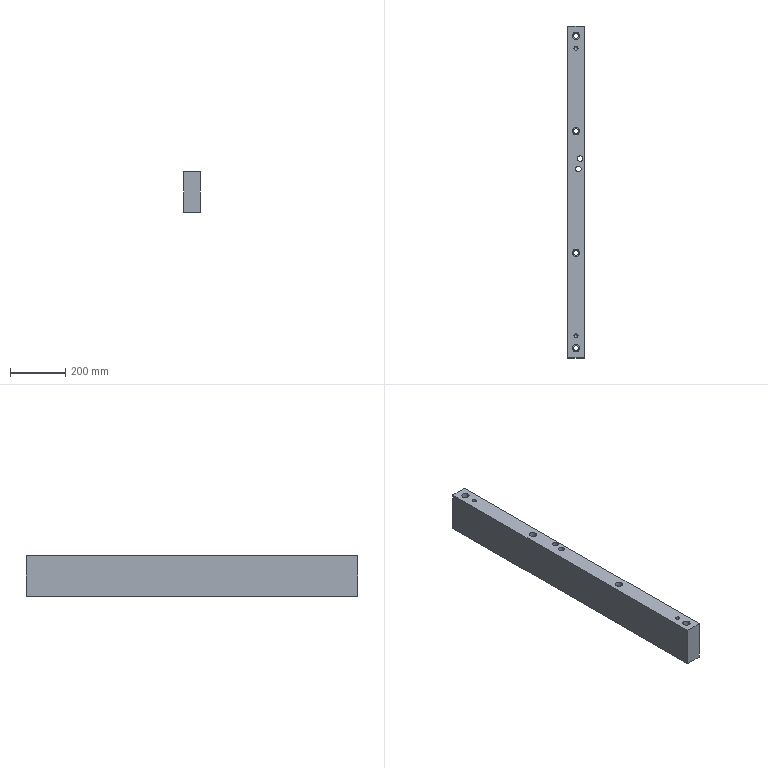Part | STEP file | lll_id2474_x_t | 1 solid | 24 faces | box 60 x 1200 x 147.5 mm | volume 10289095 mm3 | cylinder 12 | plane 10 | cone 2 | commonest cylinder face diameters 18.009 x4 26.008 x4 14.506 x2 20 x2
STEP:
#1=CARTESIAN_POINT('',(777.004,120.5,222.5));
#2=VERTEX_POINT('',#1);
#3=CARTESIAN_POINT('',(767.004,120.5,222.5));
#4=DIRECTION('',(0.,0.,1.));
#5=DIRECTION('',(1.,0.,0.));
#6=AXIS2_PLACEMENT_3D('',#3,#4,#5);
#7=CIRCLE('',#6,10.);
#8=EDGE_CURVE('',#2,#2,#7,.T.);
#9=ORIENTED_EDGE('',*,*,#8,.T.);
#10=EDGE_LOOP('',(#9));
#11=FACE_BOUND('',#10,.T.);
#12=CARTESIAN_POINT('',(761.44,-220.,222.5));
#13=VERTEX_POINT('',#12);
#14=CARTESIAN_POINT('',(752.435,-220.,222.5));
#15=DIRECTION('',(0.,0.,1.));
#16=DIRECTION('',(1.,0.,0.));
#17=AXIS2_PLACEMENT_3D('',#14,#15,#16);
#18=CIRCLE('',#17,9.005);
#19=EDGE_CURVE('',#13,#13,#18,.T.);
#20=ORIENTED_EDGE('',*,*,#19,.T.);
#21=EDGE_LOOP('',(#20));
#22=FACE_BOUND('',#21,.T.);
#23=CARTESIAN_POINT('',(722.435,600.,222.5));
#24=VERTEX_POINT('',#23);
#25=CARTESIAN_POINT('',(782.435,600.,222.5));
#26=VERTEX_POINT('',#25);
#27=CARTESIAN_POINT('',(-3187.565,600.,222.5));
#28=DIRECTION('',(1.,0.,0.));
#29=VECTOR('',#28,1.);
#30=LINE('',#27,#29);
#31=EDGE_CURVE('',#24,#26,#30,.T.);
#32=ORIENTED_EDGE('',*,*,#31,.T.);
#33=CARTESIAN_POINT('',(782.435,-600.,222.5));
#34=VERTEX_POINT('',#33);
#35=CARTESIAN_POINT('',(782.435,600.,222.5));
#36=DIRECTION('',(0.,-1.,0.));
#37=VECTOR('',#36,1.);
#38=LINE('',#35,#37);
#39=EDGE_CURVE('',#26,#34,#38,.T.);
#40=ORIENTED_EDGE('',*,*,#39,.T.);
#41=CARTESIAN_POINT('',(722.435,-600.,222.5));
#42=VERTEX_POINT('',#41);
#43=CARTESIAN_POINT('',(782.435,-600.,222.5));
#44=DIRECTION('',(-1.,0.,0.));
#45=VECTOR('',#44,1.);
#46=LINE('',#43,#45);
#47=EDGE_CURVE('',#34,#42,#46,.T.);
#48=ORIENTED_EDGE('',*,*,#47,.T.);
#49=CARTESIAN_POINT('',(722.435,1.,222.5));
#50=DIRECTION('',(0.,-1.,0.));
#51=VECTOR('',#50,1.);
#52=LINE('',#49,#51);
#53=EDGE_CURVE('',#24,#42,#52,.T.);
#54=ORIENTED_EDGE('',*,*,#53,.F.);
#55=EDGE_LOOP('',(#32,#40,#48,#54));
#56=FACE_BOUND('',#55,.T.);
#57=CARTESIAN_POINT('',(761.44,-565.,222.5));
#58=VERTEX_POINT('',#57);
#59=CARTESIAN_POINT('',(752.435,-565.,222.5));
#60=DIRECTION('',(0.,0.,1.));
#61=DIRECTION('',(1.,0.,0.));
#62=AXIS2_PLACEMENT_3D('',#59,#60,#61);
#63=CIRCLE('',#62,9.005);
#64=EDGE_CURVE('',#58,#58,#63,.T.);
#65=ORIENTED_EDGE('',*,*,#64,.T.);
#66=EDGE_LOOP('',(#65));
#67=FACE_BOUND('',#66,.T.);
#68=CARTESIAN_POINT('',(761.44,220.,222.5));
#69=VERTEX_POINT('',#68);
#70=CARTESIAN_POINT('',(752.435,220.,222.5));
#71=DIRECTION('',(0.,0.,-1.));
#72=DIRECTION('',(1.,0.,0.));
#73=AXIS2_PLACEMENT_3D('',#70,#71,#72);
#74=CIRCLE('',#73,9.005);
#75=EDGE_CURVE('',#69,#69,#74,.T.);
#76=ORIENTED_EDGE('',*,*,#75,.F.);
#77=EDGE_LOOP('',(#76));
#78=FACE_BOUND('',#77,.T.);
#79=CARTESIAN_POINT('',(761.44,565.,222.5));
#80=VERTEX_POINT('',#79);
#81=CARTESIAN_POINT('',(752.435,565.,222.5));
#82=DIRECTION('',(0.,0.,-1.));
#83=DIRECTION('',(1.,0.,0.));
#84=AXIS2_PLACEMENT_3D('',#81,#82,#83);
#85=CIRCLE('',#84,9.005);
#86=EDGE_CURVE('',#80,#80,#85,.T.);
#87=ORIENTED_EDGE('',*,*,#86,.F.);
#88=EDGE_LOOP('',(#87));
#89=FACE_BOUND('',#88,.T.);
#90=CARTESIAN_POINT('',(771.004,83.5,222.5));
#91=VERTEX_POINT('',#90);
#92=CARTESIAN_POINT('',(761.004,83.5,222.5));
#93=DIRECTION('',(0.,0.,1.));
#94=DIRECTION('',(1.,0.,0.));
#95=AXIS2_PLACEMENT_3D('',#92,#93,#94);
#96=CIRCLE('',#95,10.);
#97=EDGE_CURVE('',#91,#91,#96,.T.);
#98=ORIENTED_EDGE('',*,*,#97,.T.);
#99=EDGE_LOOP('',(#98));
#100=FACE_BOUND('',#99,.T.);
#101=CARTESIAN_POINT('',(2968.751,1.,222.5));
#102=DIRECTION('',(0.,0.,-1.));
#103=DIRECTION('',(-1.,0.,0.));
#104=AXIS2_PLACEMENT_3D('',#101,#102,#103);
#105=PLANE('',#104);
#106=ADVANCED_FACE('',(#11,#22,#56,#67,#78,#89,#100),#105,.T.);
#107=CARTESIAN_POINT('',(751.004,83.5,370.));
#108=VERTEX_POINT('',#107);
#109=CARTESIAN_POINT('',(761.004,83.5,370.));
#110=DIRECTION('',(0.,0.,-1.));
#111=DIRECTION('',(-1.,0.,0.));
#112=AXIS2_PLACEMENT_3D('',#109,#110,#111);
#113=CIRCLE('',#112,10.);
#114=EDGE_CURVE('',#108,#108,#113,.T.);
#115=ORIENTED_EDGE('',*,*,#114,.T.);
#116=EDGE_LOOP('',(#115));
#117=FACE_BOUND('',#116,.T.);
#118=CARTESIAN_POINT('',(757.004,120.5,370.));
#119=VERTEX_POINT('',#118);
#120=CARTESIAN_POINT('',(767.004,120.5,370.));
#121=DIRECTION('',(0.,0.,-1.));
#122=DIRECTION('',(-1.,0.,0.));
#123=AXIS2_PLACEMENT_3D('',#120,#121,#122);
#124=CIRCLE('',#123,10.);
#125=EDGE_CURVE('',#119,#119,#124,.T.);
#126=ORIENTED_EDGE('',*,*,#125,.T.);
#127=EDGE_LOOP('',(#126));
#128=FACE_BOUND('',#127,.T.);
#129=CARTESIAN_POINT('',(759.688,-520.,370.));
#130=VERTEX_POINT('',#129);
#131=CARTESIAN_POINT('',(752.435,-520.,370.));
#132=DIRECTION('',(0.,0.,-1.));
#133=DIRECTION('',(1.,0.,0.));
#134=AXIS2_PLACEMENT_3D('',#131,#132,#133);
#135=CIRCLE('',#134,7.253);
#136=EDGE_CURVE('',#130,#130,#135,.T.);
#137=ORIENTED_EDGE('',*,*,#136,.T.);
#138=EDGE_LOOP('',(#137));
#139=FACE_BOUND('',#138,.T.);
#140=CARTESIAN_POINT('',(759.688,520.,370.));
#141=VERTEX_POINT('',#140);
#142=CARTESIAN_POINT('',(752.435,520.,370.));
#143=DIRECTION('',(0.,0.,1.));
#144=DIRECTION('',(1.,0.,0.));
#145=AXIS2_PLACEMENT_3D('',#142,#143,#144);
#146=CIRCLE('',#145,7.253);
#147=EDGE_CURVE('',#141,#141,#146,.T.);
#148=ORIENTED_EDGE('',*,*,#147,.F.);
#149=EDGE_LOOP('',(#148));
#150=FACE_BOUND('',#149,.T.);
#151=CARTESIAN_POINT('',(765.439,565.,370.));
#152=VERTEX_POINT('',#151);
#153=CARTESIAN_POINT('',(752.435,565.,370.));
#154=DIRECTION('',(0.,0.,1.));
#155=DIRECTION('',(1.,0.,0.));
#156=AXIS2_PLACEMENT_3D('',#153,#154,#155);
#157=CIRCLE('',#156,13.004);
#158=EDGE_CURVE('',#152,#152,#157,.T.);
#159=ORIENTED_EDGE('',*,*,#158,.F.);
#160=EDGE_LOOP('',(#159));
#161=FACE_BOUND('',#160,.T.);
#162=CARTESIAN_POINT('',(722.435,600.,370.));
#163=VERTEX_POINT('',#162);
#164=CARTESIAN_POINT('',(782.435,600.,370.));
#165=VERTEX_POINT('',#164);
#166=CARTESIAN_POINT('',(2968.751,600.,370.));
#167=DIRECTION('',(1.,0.,0.));
#168=VECTOR('',#167,1.);
#169=LINE('',#166,#168);
#170=EDGE_CURVE('',#163,#165,#169,.T.);
#171=ORIENTED_EDGE('',*,*,#170,.F.);
#172=CARTESIAN_POINT('',(722.435,-600.,370.));
#173=VERTEX_POINT('',#172);
#174=CARTESIAN_POINT('',(722.435,0.,370.));
#175=DIRECTION('',(0.,1.,0.));
#176=VECTOR('',#175,1.);
#177=LINE('',#174,#176);
#178=EDGE_CURVE('',#173,#163,#177,.T.);
#179=ORIENTED_EDGE('',*,*,#178,.F.);
#180=CARTESIAN_POINT('',(782.435,-600.,370.));
#181=VERTEX_POINT('',#180);
#182=CARTESIAN_POINT('',(2968.751,-600.,370.));
#183=DIRECTION('',(-1.,0.,0.));
#184=VECTOR('',#183,1.);
#185=LINE('',#182,#184);
#186=EDGE_CURVE('',#181,#173,#185,.T.);
#187=ORIENTED_EDGE('',*,*,#186,.F.);
#188=CARTESIAN_POINT('',(782.435,1.,370.));
#189=DIRECTION('',(0.,-1.,0.));
#190=VECTOR('',#189,1.);
#191=LINE('',#188,#190);
#192=EDGE_CURVE('',#165,#181,#191,.T.);
#193=ORIENTED_EDGE('',*,*,#192,.F.);
#194=EDGE_LOOP('',(#171,#179,#187,#193));
#195=FACE_BOUND('',#194,.T.);
#196=CARTESIAN_POINT('',(765.439,-565.,370.));
#197=VERTEX_POINT('',#196);
#198=CARTESIAN_POINT('',(752.435,-565.,370.));
#199=DIRECTION('',(0.,0.,-1.));
#200=DIRECTION('',(1.,0.,0.));
#201=AXIS2_PLACEMENT_3D('',#198,#199,#200);
#202=CIRCLE('',#201,13.004);
#203=EDGE_CURVE('',#197,#197,#202,.T.);
#204=ORIENTED_EDGE('',*,*,#203,.T.);
#205=EDGE_LOOP('',(#204));
#206=FACE_BOUND('',#205,.T.);
#207=CARTESIAN_POINT('',(765.439,-220.,370.));
#208=VERTEX_POINT('',#207);
#209=CARTESIAN_POINT('',(752.435,-220.,370.));
#210=DIRECTION('',(0.,0.,-1.));
#211=DIRECTION('',(1.,0.,0.));
#212=AXIS2_PLACEMENT_3D('',#209,#210,#211);
#213=CIRCLE('',#212,13.004);
#214=EDGE_CURVE('',#208,#208,#213,.T.);
#215=ORIENTED_EDGE('',*,*,#214,.T.);
#216=EDGE_LOOP('',(#215));
#217=FACE_BOUND('',#216,.T.);
#218=CARTESIAN_POINT('',(765.439,220.,370.));
#219=VERTEX_POINT('',#218);
#220=CARTESIAN_POINT('',(752.435,220.,370.));
#221=DIRECTION('',(0.,0.,1.));
#222=DIRECTION('',(1.,0.,0.));
#223=AXIS2_PLACEMENT_3D('',#220,#221,#222);
#224=CIRCLE('',#223,13.004);
#225=EDGE_CURVE('',#219,#219,#224,.T.);
#226=ORIENTED_EDGE('',*,*,#225,.F.);
#227=EDGE_LOOP('',(#226));
#228=FACE_BOUND('',#227,.T.);
#229=CARTESIAN_POINT('',(2968.751,1.,370.));
#230=DIRECTION('',(0.,0.,-1.));
#231=DIRECTION('',(-1.,0.,0.));
#232=AXIS2_PLACEMENT_3D('',#229,#230,#231);
#233=PLANE('',#232);
#234=ADVANCED_FACE('',(#117,#128,#139,#150,#161,#195,#206,#217,#228),#233,.F.);
#235=ORIENTED_EDGE('',*,*,#39,.F.);
#236=CARTESIAN_POINT('',(782.435,600.,360.));
#237=DIRECTION('',(0.,0.,-1.));
#238=VECTOR('',#237,1.);
#239=LINE('',#236,#238);
#240=EDGE_CURVE('',#165,#26,#239,.T.);
#241=ORIENTED_EDGE('',*,*,#240,.F.);
#242=ORIENTED_EDGE('',*,*,#192,.T.);
#243=CARTESIAN_POINT('',(782.435,-600.,360.));
#244=DIRECTION('',(0.,0.,-1.));
#245=VECTOR('',#244,1.);
#246=LINE('',#243,#245);
#247=EDGE_CURVE('',#181,#34,#246,.T.);
#248=ORIENTED_EDGE('',*,*,#247,.T.);
#249=EDGE_LOOP('',(#235,#241,#242,#248));
#250=FACE_OUTER_BOUND('',#249,.T.);
#251=CARTESIAN_POINT('',(782.435,600.,360.));
#252=DIRECTION('',(1.,0.,0.));
#253=DIRECTION('',(0.,0.,-1.));
#254=AXIS2_PLACEMENT_3D('',#251,#252,#253);
#255=PLANE('',#254);
#256=ADVANCED_FACE('',(#250),#255,.T.);
#257=CARTESIAN_POINT('',(722.435,-600.,360.));
#258=DIRECTION('',(0.,0.,-1.));
#259=VECTOR('',#258,1.);
#260=LINE('',#257,#259);
#261=EDGE_CURVE('',#173,#42,#260,.T.);
#262=ORIENTED_EDGE('',*,*,#261,.T.);
#263=ORIENTED_EDGE('',*,*,#47,.F.);
#264=ORIENTED_EDGE('',*,*,#247,.F.);
#265=ORIENTED_EDGE('',*,*,#186,.T.);
#266=EDGE_LOOP('',(#262,#263,#264,#265));
#267=FACE_OUTER_BOUND('',#266,.T.);
#268=CARTESIAN_POINT('',(782.435,-600.,360.));
#269=DIRECTION('',(0.,-1.,0.));
#270=DIRECTION('',(0.,0.,-1.));
#271=AXIS2_PLACEMENT_3D('',#268,#269,#270);
#272=PLANE('',#271);
#273=ADVANCED_FACE('',(#267),#272,.T.);
#274=CARTESIAN_POINT('',(722.435,600.,360.));
#275=DIRECTION('',(0.,0.,1.));
#276=VECTOR('',#275,1.);
#277=LINE('',#274,#276);
#278=EDGE_CURVE('',#24,#163,#277,.T.);
#279=ORIENTED_EDGE('',*,*,#278,.T.);
#280=ORIENTED_EDGE('',*,*,#170,.T.);
#281=ORIENTED_EDGE('',*,*,#240,.T.);
#282=ORIENTED_EDGE('',*,*,#31,.F.);
#283=EDGE_LOOP('',(#279,#280,#281,#282));
#284=FACE_OUTER_BOUND('',#283,.T.);
#285=CARTESIAN_POINT('',(-3187.565,600.,360.));
#286=DIRECTION('',(0.,1.,0.));
#287=DIRECTION('',(0.,0.,1.));
#288=AXIS2_PLACEMENT_3D('',#285,#286,#287);
#289=PLANE('',#288);
#290=ADVANCED_FACE('',(#284),#289,.T.);
#291=ORIENTED_EDGE('',*,*,#53,.T.);
#292=ORIENTED_EDGE('',*,*,#261,.F.);
#293=ORIENTED_EDGE('',*,*,#178,.T.);
#294=ORIENTED_EDGE('',*,*,#278,.F.);
#295=EDGE_LOOP('',(#291,#292,#293,#294));
#296=FACE_OUTER_BOUND('',#295,.T.);
#297=CARTESIAN_POINT('',(722.435,0.,291.25));
#298=DIRECTION('',(1.,0.,0.));
#299=DIRECTION('',(0.,0.,-1.));
#300=AXIS2_PLACEMENT_3D('',#297,#298,#299);
#301=PLANE('',#300);
#302=ADVANCED_FACE('',(#296),#301,.F.);
#303=CARTESIAN_POINT('',(743.431,-565.,302.5));
#304=VERTEX_POINT('',#303);
#305=CARTESIAN_POINT('',(752.435,-565.,302.5));
#306=DIRECTION('',(0.,0.,-1.));
#307=DIRECTION('',(-1.,0.,0.));
#308=AXIS2_PLACEMENT_3D('',#305,#306,#307);
#309=CIRCLE('',#308,9.005);
#310=EDGE_CURVE('',#304,#304,#309,.T.);
#311=ORIENTED_EDGE('',*,*,#310,.F.);
#312=EDGE_LOOP('',(#311));
#313=FACE_BOUND('',#312,.T.);
#314=ORIENTED_EDGE('',*,*,#64,.F.);
#315=EDGE_LOOP('',(#314));
#316=FACE_BOUND('',#315,.T.);
#317=CARTESIAN_POINT('',(752.435,-565.,420.));
#318=DIRECTION('',(0.,0.,-1.));
#319=DIRECTION('',(1.,0.,0.));
#320=AXIS2_PLACEMENT_3D('',#317,#318,#319);
#321=CYLINDRICAL_SURFACE('',#320,9.005);
#322=ADVANCED_FACE('',(#313,#316),#321,.F.);
#323=ORIENTED_EDGE('',*,*,#310,.T.);
#324=EDGE_LOOP('',(#323));
#325=FACE_BOUND('',#324,.T.);
#326=CARTESIAN_POINT('',(765.439,-565.,302.5));
#327=VERTEX_POINT('',#326);
#328=CARTESIAN_POINT('',(752.435,-565.,302.5));
#329=DIRECTION('',(0.,0.,-1.));
#330=DIRECTION('',(-1.,0.,0.));
#331=AXIS2_PLACEMENT_3D('',#328,#329,#330);
#332=CIRCLE('',#331,13.004);
#333=EDGE_CURVE('',#327,#327,#332,.T.);
#334=ORIENTED_EDGE('',*,*,#333,.F.);
#335=EDGE_LOOP('',(#334));
#336=FACE_BOUND('',#335,.T.);
#337=CARTESIAN_POINT('',(752.435,-565.,302.5));
#338=DIRECTION('',(0.,0.,-1.));
#339=DIRECTION('',(-1.,0.,0.));
#340=AXIS2_PLACEMENT_3D('',#337,#338,#339);
#341=PLANE('',#340);
#342=ADVANCED_FACE('',(#325,#336),#341,.F.);
#343=ORIENTED_EDGE('',*,*,#333,.T.);
#344=EDGE_LOOP('',(#343));
#345=FACE_BOUND('',#344,.T.);
#346=ORIENTED_EDGE('',*,*,#203,.F.);
#347=EDGE_LOOP('',(#346));
#348=FACE_BOUND('',#347,.T.);
#349=CARTESIAN_POINT('',(752.435,-565.,420.));
#350=DIRECTION('',(0.,0.,-1.));
#351=DIRECTION('',(1.,0.,0.));
#352=AXIS2_PLACEMENT_3D('',#349,#350,#351);
#353=CYLINDRICAL_SURFACE('',#352,13.004);
#354=ADVANCED_FACE('',(#345,#348),#353,.F.);
#355=CARTESIAN_POINT('',(743.431,-220.,302.5));
#356=VERTEX_POINT('',#355);
#357=CARTESIAN_POINT('',(752.435,-220.,302.5));
#358=DIRECTION('',(0.,0.,-1.));
#359=DIRECTION('',(-1.,0.,0.));
#360=AXIS2_PLACEMENT_3D('',#357,#358,#359);
#361=CIRCLE('',#360,9.005);
#362=EDGE_CURVE('',#356,#356,#361,.T.);
#363=ORIENTED_EDGE('',*,*,#362,.F.);
#364=EDGE_LOOP('',(#363));
#365=FACE_BOUND('',#364,.T.);
#366=ORIENTED_EDGE('',*,*,#19,.F.);
#367=EDGE_LOOP('',(#366));
#368=FACE_BOUND('',#367,.T.);
#369=CARTESIAN_POINT('',(752.435,-220.,420.));
#370=DIRECTION('',(0.,0.,-1.));
#371=DIRECTION('',(1.,0.,0.));
#372=AXIS2_PLACEMENT_3D('',#369,#370,#371);
#373=CYLINDRICAL_SURFACE('',#372,9.005);
#374=ADVANCED_FACE('',(#365,#368),#373,.F.);
#375=ORIENTED_EDGE('',*,*,#362,.T.);
#376=EDGE_LOOP('',(#375));
#377=FACE_BOUND('',#376,.T.);
#378=CARTESIAN_POINT('',(765.439,-220.,302.5));
#379=VERTEX_POINT('',#378);
#380=CARTESIAN_POINT('',(752.435,-220.,302.5));
#381=DIRECTION('',(0.,0.,-1.));
#382=DIRECTION('',(1.,0.,0.));
#383=AXIS2_PLACEMENT_3D('',#380,#381,#382);
#384=CIRCLE('',#383,13.004);
#385=EDGE_CURVE('',#379,#379,#384,.T.);
#386=ORIENTED_EDGE('',*,*,#385,.F.);
#387=EDGE_LOOP('',(#386));
#388=FACE_BOUND('',#387,.T.);
#389=CARTESIAN_POINT('',(752.435,-220.,302.5));
#390=DIRECTION('',(0.,0.,-1.));
#391=DIRECTION('',(-1.,0.,0.));
#392=AXIS2_PLACEMENT_3D('',#389,#390,#391);
#393=PLANE('',#392);
#394=ADVANCED_FACE('',(#377,#388),#393,.F.);
#395=ORIENTED_EDGE('',*,*,#385,.T.);
#396=EDGE_LOOP('',(#395));
#397=FACE_BOUND('',#396,.T.);
#398=ORIENTED_EDGE('',*,*,#214,.F.);
#399=EDGE_LOOP('',(#398));
#400=FACE_BOUND('',#399,.T.);
#401=CARTESIAN_POINT('',(752.435,-220.,420.));
#402=DIRECTION('',(0.,0.,-1.));
#403=DIRECTION('',(1.,0.,0.));
#404=AXIS2_PLACEMENT_3D('',#401,#402,#403);
#405=CYLINDRICAL_SURFACE('',#404,13.004);
#406=ADVANCED_FACE('',(#397,#400),#405,.F.);
#407=CARTESIAN_POINT('',(743.431,220.,302.5));
#408=VERTEX_POINT('',#407);
#409=CARTESIAN_POINT('',(752.435,220.,302.5));
#410=DIRECTION('',(0.,0.,1.));
#411=DIRECTION('',(-1.,0.,0.));
#412=AXIS2_PLACEMENT_3D('',#409,#410,#411);
#413=CIRCLE('',#412,9.005);
#414=EDGE_CURVE('',#408,#408,#413,.T.);
#415=ORIENTED_EDGE('',*,*,#414,.T.);
#416=EDGE_LOOP('',(#415));
#417=FACE_BOUND('',#416,.T.);
#418=ORIENTED_EDGE('',*,*,#75,.T.);
#419=EDGE_LOOP('',(#418));
#420=FACE_BOUND('',#419,.T.);
#421=CARTESIAN_POINT('',(752.435,220.,420.));
#422=DIRECTION('',(0.,0.,-1.));
#423=DIRECTION('',(1.,0.,0.));
#424=AXIS2_PLACEMENT_3D('',#421,#422,#423);
#425=CYLINDRICAL_SURFACE('',#424,9.005);
#426=ADVANCED_FACE('',(#417,#420),#425,.F.);
#427=ORIENTED_EDGE('',*,*,#414,.F.);
#428=EDGE_LOOP('',(#427));
#429=FACE_BOUND('',#428,.T.);
#430=CARTESIAN_POINT('',(765.439,220.,302.5));
#431=VERTEX_POINT('',#430);
#432=CARTESIAN_POINT('',(752.435,220.,302.5));
#433=DIRECTION('',(0.,0.,1.));
#434=DIRECTION('',(1.,0.,0.));
#435=AXIS2_PLACEMENT_3D('',#432,#433,#434);
#436=CIRCLE('',#435,13.004);
#437=EDGE_CURVE('',#431,#431,#436,.T.);
#438=ORIENTED_EDGE('',*,*,#437,.T.);
#439=EDGE_LOOP('',(#438));
#440=FACE_BOUND('',#439,.T.);
#441=CARTESIAN_POINT('',(752.435,220.,302.5));
#442=DIRECTION('',(0.,0.,-1.));
#443=DIRECTION('',(-1.,0.,0.));
#444=AXIS2_PLACEMENT_3D('',#441,#442,#443);
#445=PLANE('',#444);
#446=ADVANCED_FACE('',(#429,#440),#445,.F.);
#447=ORIENTED_EDGE('',*,*,#437,.F.);
#448=EDGE_LOOP('',(#447));
#449=FACE_BOUND('',#448,.T.);
#450=ORIENTED_EDGE('',*,*,#225,.T.);
#451=EDGE_LOOP('',(#450));
#452=FACE_BOUND('',#451,.T.);
#453=CARTESIAN_POINT('',(752.435,220.,420.));
#454=DIRECTION('',(0.,0.,-1.));
#455=DIRECTION('',(1.,0.,0.));
#456=AXIS2_PLACEMENT_3D('',#453,#454,#455);
#457=CYLINDRICAL_SURFACE('',#456,13.004);
#458=ADVANCED_FACE('',(#449,#452),#457,.F.);
#459=CARTESIAN_POINT('',(743.431,565.,302.5));
#460=VERTEX_POINT('',#459);
#461=CARTESIAN_POINT('',(752.435,565.,302.5));
#462=DIRECTION('',(0.,0.,1.));
#463=DIRECTION('',(-1.,0.,0.));
#464=AXIS2_PLACEMENT_3D('',#461,#462,#463);
#465=CIRCLE('',#464,9.005);
#466=EDGE_CURVE('',#460,#460,#465,.T.);
#467=ORIENTED_EDGE('',*,*,#466,.T.);
#468=EDGE_LOOP('',(#467));
#469=FACE_BOUND('',#468,.T.);
#470=ORIENTED_EDGE('',*,*,#86,.T.);
#471=EDGE_LOOP('',(#470));
#472=FACE_BOUND('',#471,.T.);
#473=CARTESIAN_POINT('',(752.435,565.,420.));
#474=DIRECTION('',(0.,0.,-1.));
#475=DIRECTION('',(1.,0.,0.));
#476=AXIS2_PLACEMENT_3D('',#473,#474,#475);
#477=CYLINDRICAL_SURFACE('',#476,9.005);
#478=ADVANCED_FACE('',(#469,#472),#477,.F.);
#479=ORIENTED_EDGE('',*,*,#466,.F.);
#480=EDGE_LOOP('',(#479));
#481=FACE_BOUND('',#480,.T.);
#482=CARTESIAN_POINT('',(765.439,565.,302.5));
#483=VERTEX_POINT('',#482);
#484=CARTESIAN_POINT('',(752.435,565.,302.5));
#485=DIRECTION('',(0.,0.,1.));
#486=DIRECTION('',(1.,0.,0.));
#487=AXIS2_PLACEMENT_3D('',#484,#485,#486);
#488=CIRCLE('',#487,13.004);
#489=EDGE_CURVE('',#483,#483,#488,.T.);
#490=ORIENTED_EDGE('',*,*,#489,.T.);
#491=EDGE_LOOP('',(#490));
#492=FACE_BOUND('',#491,.T.);
#493=CARTESIAN_POINT('',(752.435,565.,302.5));
#494=DIRECTION('',(0.,0.,-1.));
#495=DIRECTION('',(-1.,0.,0.));
#496=AXIS2_PLACEMENT_3D('',#493,#494,#495);
#497=PLANE('',#496);
#498=ADVANCED_FACE('',(#481,#492),#497,.F.);
#499=ORIENTED_EDGE('',*,*,#489,.F.);
#500=EDGE_LOOP('',(#499));
#501=FACE_BOUND('',#500,.T.);
#502=ORIENTED_EDGE('',*,*,#158,.T.);
#503=EDGE_LOOP('',(#502));
#504=FACE_BOUND('',#503,.T.);
#505=CARTESIAN_POINT('',(752.435,565.,420.));
#506=DIRECTION('',(0.,0.,-1.));
#507=DIRECTION('',(1.,0.,0.));
#508=AXIS2_PLACEMENT_3D('',#505,#506,#507);
#509=CYLINDRICAL_SURFACE('',#508,13.004);
#510=ADVANCED_FACE('',(#501,#504),#509,.F.);
#511=CARTESIAN_POINT('',(745.182,520.,332.247));
#512=VERTEX_POINT('',#511);
#513=CARTESIAN_POINT('',(752.435,520.,332.247));
#514=DIRECTION('',(0.,0.,1.));
#515=DIRECTION('',(-1.,0.,0.));
#516=AXIS2_PLACEMENT_3D('',#513,#514,#515);
#517=CIRCLE('',#516,7.253);
#518=EDGE_CURVE('',#512,#512,#517,.T.);
#519=ORIENTED_EDGE('',*,*,#518,.F.);
#520=EDGE_LOOP('',(#519));
#521=FACE_BOUND('',#520,.T.);
#522=ORIENTED_EDGE('',*,*,#147,.T.);
#523=EDGE_LOOP('',(#522));
#524=FACE_BOUND('',#523,.T.);
#525=CARTESIAN_POINT('',(752.435,520.,370.));
#526=DIRECTION('',(0.,0.,-1.));
#527=DIRECTION('',(1.,0.,0.));
#528=AXIS2_PLACEMENT_3D('',#525,#526,#527);
#529=CYLINDRICAL_SURFACE('',#528,7.253);
#530=ADVANCED_FACE('',(#521,#524),#529,.F.);
#531=CARTESIAN_POINT('',(752.435,520.,324.994));
#532=VERTEX_POINT('',#531);
#533=VERTEX_LOOP('',#532);
#534=FACE_BOUND('',#533,.T.);
#535=ORIENTED_EDGE('',*,*,#518,.T.);
#536=EDGE_LOOP('',(#535));
#537=FACE_BOUND('',#536,.T.);
#538=CARTESIAN_POINT('',(752.435,520.,332.247));
#539=DIRECTION('',(0.,0.,1.));
#540=DIRECTION('',(1.,0.,0.));
#541=AXIS2_PLACEMENT_3D('',#538,#539,#540);
#542=CONICAL_SURFACE('',#541,7.253,45.);
#543=ADVANCED_FACE('',(#534,#537),#542,.F.);
#544=CARTESIAN_POINT('',(745.182,-520.,332.247));
#545=VERTEX_POINT('',#544);
#546=CARTESIAN_POINT('',(752.435,-520.,332.247));
#547=DIRECTION('',(0.,0.,-1.));
#548=DIRECTION('',(-1.,0.,0.));
#549=AXIS2_PLACEMENT_3D('',#546,#547,#548);
#550=CIRCLE('',#549,7.253);
#551=EDGE_CURVE('',#545,#545,#550,.T.);
#552=ORIENTED_EDGE('',*,*,#551,.T.);
#553=EDGE_LOOP('',(#552));
#554=FACE_BOUND('',#553,.T.);
#555=ORIENTED_EDGE('',*,*,#136,.F.);
#556=EDGE_LOOP('',(#555));
#557=FACE_BOUND('',#556,.T.);
#558=CARTESIAN_POINT('',(752.435,-520.,370.));
#559=DIRECTION('',(0.,0.,-1.));
#560=DIRECTION('',(1.,0.,0.));
#561=AXIS2_PLACEMENT_3D('',#558,#559,#560);
#562=CYLINDRICAL_SURFACE('',#561,7.253);
#563=ADVANCED_FACE('',(#554,#557),#562,.F.);
#564=CARTESIAN_POINT('',(752.435,-520.,324.994));
#565=VERTEX_POINT('',#564);
#566=VERTEX_LOOP('',#565);
#567=FACE_BOUND('',#566,.T.);
#568=ORIENTED_EDGE('',*,*,#551,.F.);
#569=EDGE_LOOP('',(#568));
#570=FACE_BOUND('',#569,.T.);
#571=CARTESIAN_POINT('',(752.435,-520.,332.247));
#572=DIRECTION('',(0.,0.,1.));
#573=DIRECTION('',(1.,0.,0.));
#574=AXIS2_PLACEMENT_3D('',#571,#572,#573);
#575=CONICAL_SURFACE('',#574,7.253,45.);
#576=ADVANCED_FACE('',(#567,#570),#575,.F.);
#577=ORIENTED_EDGE('',*,*,#8,.F.);
#578=EDGE_LOOP('',(#577));
#579=FACE_BOUND('',#578,.T.);
#580=ORIENTED_EDGE('',*,*,#125,.F.);
#581=EDGE_LOOP('',(#580));
#582=FACE_BOUND('',#581,.T.);
#583=CARTESIAN_POINT('',(767.004,120.5,222.5));
#584=DIRECTION('',(0.,0.,1.));
#585=DIRECTION('',(-1.,0.,0.));
#586=AXIS2_PLACEMENT_3D('',#583,#584,#585);
#587=CYLINDRICAL_SURFACE('',#586,10.);
#588=ADVANCED_FACE('',(#579,#582),#587,.F.);
#589=ORIENTED_EDGE('',*,*,#97,.F.);
#590=EDGE_LOOP('',(#589));
#591=FACE_BOUND('',#590,.T.);
#592=ORIENTED_EDGE('',*,*,#114,.F.);
#593=EDGE_LOOP('',(#592));
#594=FACE_BOUND('',#593,.T.);
#595=CARTESIAN_POINT('',(761.004,83.5,222.5));
#596=DIRECTION('',(0.,0.,1.));
#597=DIRECTION('',(-1.,0.,0.));
#598=AXIS2_PLACEMENT_3D('',#595,#596,#597);
#599=CYLINDRICAL_SURFACE('',#598,10.);
#600=ADVANCED_FACE('',(#591,#594),#599,.F.);
#601=CLOSED_SHELL('',(#106,#234,#256,#273,#290,#302,#322,#342,#354,#374,#394,#406,#426,#446,#458,#478,#498,#510,#530,#543,#563,#576,#588,#600));
#602=MANIFOLD_SOLID_BREP('',#601);
#603=(LENGTH_UNIT()NAMED_UNIT(*)SI_UNIT(.MILLI.,.METRE.));
#604=UNCERTAINTY_MEASURE_WITH_UNIT(LENGTH_MEASURE(0.00002),#603,'','');
#605=(NAMED_UNIT(*)PLANE_ANGLE_UNIT()SI_UNIT($,.RADIAN.));
#606=PLANE_ANGLE_MEASURE_WITH_UNIT(PLANE_ANGLE_MEASURE(0.01745),#605);
#607=DIMENSIONAL_EXPONENTS(0.,0.,0.,0.,0.,0.,0.);
#608=(CONVERSION_BASED_UNIT('DEGREE',#606)NAMED_UNIT(#607)PLANE_ANGLE_UNIT());
#609=(NAMED_UNIT(*)SI_UNIT($,.STERADIAN.)SOLID_ANGLE_UNIT());
#610=(GEOMETRIC_REPRESENTATION_CONTEXT(3)GLOBAL_UNCERTAINTY_ASSIGNED_CONTEXT((#604))GLOBAL_UNIT_ASSIGNED_CONTEXT((#603,#608,#609))REPRESENTATION_CONTEXT('',''));
#611=ADVANCED_BREP_SHAPE_REPRESENTATION('',(#602),#610);